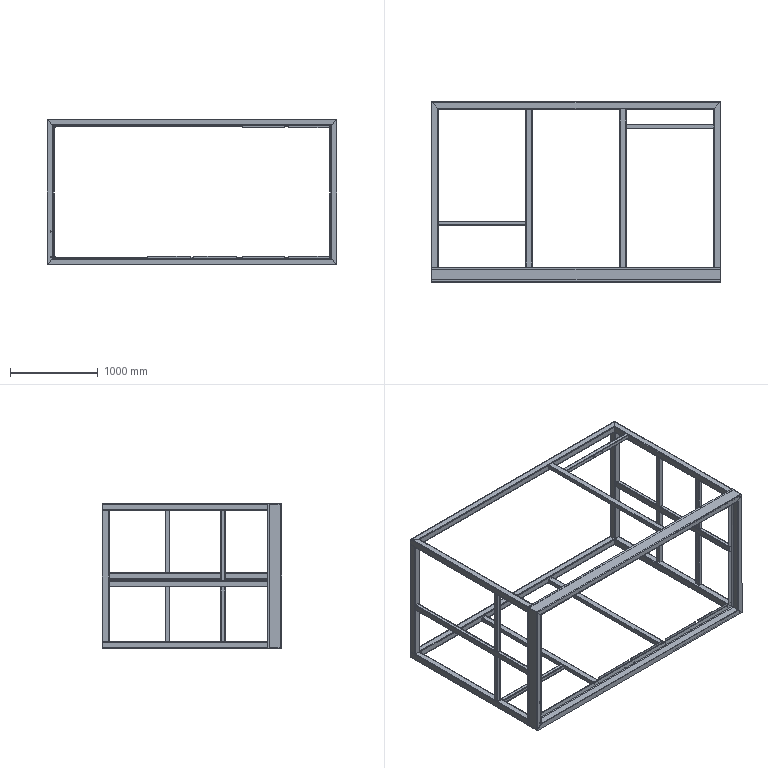Part | SolidWorks | 33 solids | 548 faces | box 3300 x 2050 x 1650 mm | volume 50652929 mm3 | plane 356 | cylinder 192 | commonest cylinder face diameters 6 x36 12 x36 8 x32 16 x32 10.5 x16 10 x10